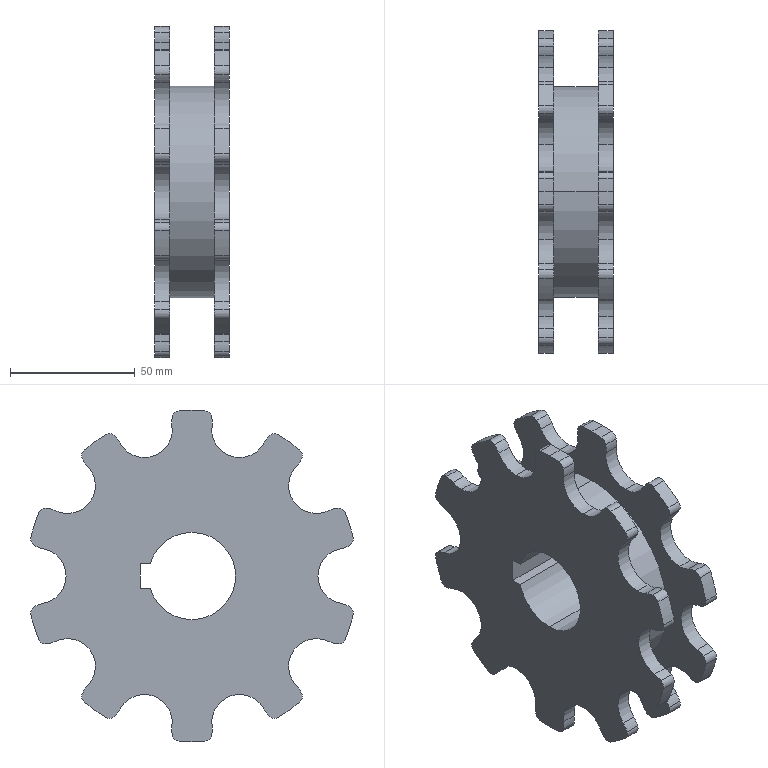Part | STEP file | PN_0003_default | 1 solid | 150 faces | box 30 x 129.474 x 133 mm | volume 202077 mm3 | cylinder 143 | plane 7 | commonest cylinder face diameters 22.23 x68 6 x48 133 x22 35 x3 85 x2